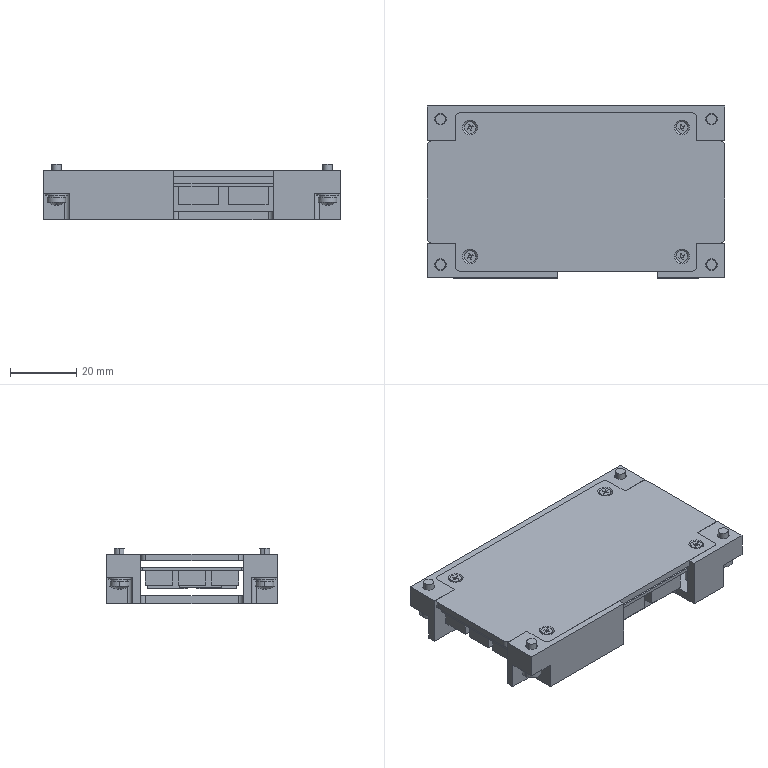Part | SolidWorks | features BaseBody 28 | 28 solids | 488 faces | box 90 x 52 x 16.8 mm | volume 31722 mm3 | plane 280 | cylinder 176 | cone 24 | spline 8 | commonest cylinder face diameters 3 x42 0.6 x32 3.2 x16 3.5 x16 2 x12 1.6 x8